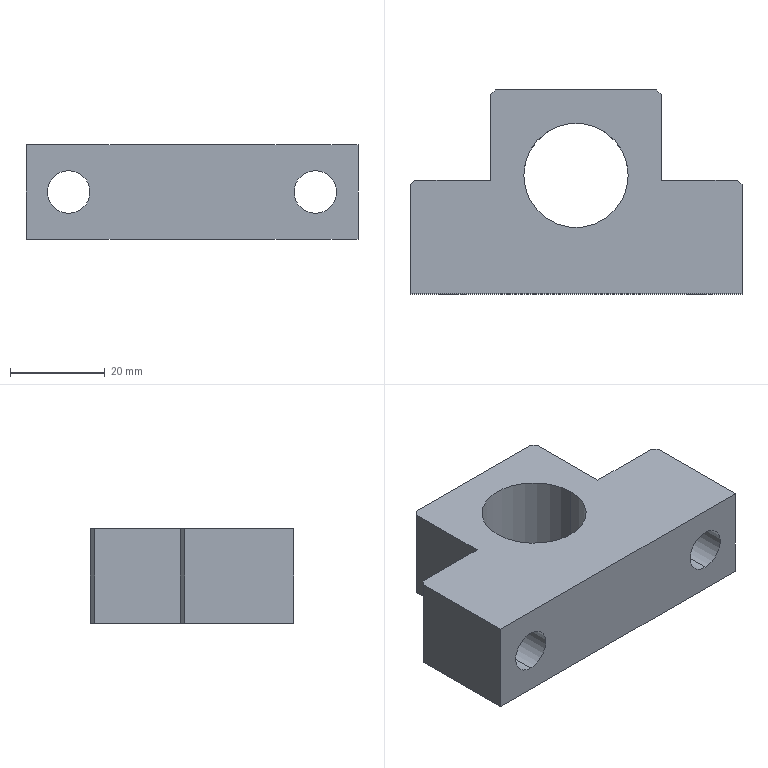Part | SolidWorks | features BaseBody 1 | 1 solid | 20 faces | box 70 x 43 x 20 mm | volume 36584 mm3 | plane 14 | cylinder 6 | commonest cylinder face diameters 9 x4 22 x2
STEP:
#1=CARTESIAN_POINT('',(-11.,0.,-10.));
#2=VERTEX_POINT('',#1);
#3=CARTESIAN_POINT('',(11.,0.,-10.));
#4=VERTEX_POINT('',#3);
#5=CARTESIAN_POINT('',(0.,0.,-10.));
#6=DIRECTION('',(0.,0.,1.));
#7=DIRECTION('',(1.,0.,0.));
#8=AXIS2_PLACEMENT_3D('',#5,#6,#7);
#9=CIRCLE('',#8,11.);
#10=EDGE_CURVE('',#2,#4,#9,.T.);
#11=ORIENTED_EDGE('',*,*,#10,.F.);
#12=CARTESIAN_POINT('',(-11.,0.,10.));
#13=VERTEX_POINT('',#12);
#14=CARTESIAN_POINT('',(-11.,0.,10.));
#15=DIRECTION('',(0.,0.,1.));
#16=VECTOR('',#15,1000.);
#17=LINE('',#14,#16);
#18=EDGE_CURVE('',#2,#13,#17,.T.);
#19=ORIENTED_EDGE('',*,*,#18,.T.);
#20=CARTESIAN_POINT('',(11.,0.,10.));
#21=VERTEX_POINT('',#20);
#22=CARTESIAN_POINT('',(0.,0.,10.));
#23=DIRECTION('',(0.,0.,1.));
#24=DIRECTION('',(1.,0.,0.));
#25=AXIS2_PLACEMENT_3D('',#22,#23,#24);
#26=CIRCLE('',#25,11.);
#27=EDGE_CURVE('',#13,#21,#26,.T.);
#28=ORIENTED_EDGE('',*,*,#27,.T.);
#29=CARTESIAN_POINT('',(11.,0.,10.));
#30=DIRECTION('',(0.,0.,1.));
#31=VECTOR('',#30,1000.);
#32=LINE('',#29,#31);
#33=EDGE_CURVE('',#4,#21,#32,.T.);
#34=ORIENTED_EDGE('',*,*,#33,.F.);
#35=EDGE_LOOP('',(#11,#19,#28,#34));
#36=FACE_OUTER_BOUND('',#35,.T.);
#37=CARTESIAN_POINT('',(0.,0.,10.));
#38=DIRECTION('',(0.,0.,1.));
#39=DIRECTION('',(1.,0.,0.));
#40=AXIS2_PLACEMENT_3D('',#37,#38,#39);
#41=CYLINDRICAL_SURFACE('',#40,11.);
#42=ADVANCED_FACE('',(#36),#41,.F.);
#43=CARTESIAN_POINT('',(26.,-25.,4.5));
#44=VERTEX_POINT('',#43);
#45=CARTESIAN_POINT('',(26.,-25.,-4.5));
#46=VERTEX_POINT('',#45);
#47=CARTESIAN_POINT('',(26.,-25.,0.));
#48=DIRECTION('',(0.,-1.,0.));
#49=DIRECTION('',(0.,0.,1.));
#50=AXIS2_PLACEMENT_3D('',#47,#48,#49);
#51=CIRCLE('',#50,4.5);
#52=EDGE_CURVE('',#44,#46,#51,.T.);
#53=ORIENTED_EDGE('',*,*,#52,.T.);
#54=CARTESIAN_POINT('',(26.,-1.,-4.5));
#55=VERTEX_POINT('',#54);
#56=CARTESIAN_POINT('',(26.,-25.,-4.5));
#57=DIRECTION('',(0.,1.,0.));
#58=VECTOR('',#57,1000.);
#59=LINE('',#56,#58);
#60=EDGE_CURVE('',#46,#55,#59,.T.);
#61=ORIENTED_EDGE('',*,*,#60,.T.);
#62=CARTESIAN_POINT('',(26.,-1.,4.5));
#63=VERTEX_POINT('',#62);
#64=CARTESIAN_POINT('',(26.,-1.,0.));
#65=DIRECTION('',(0.,1.,0.));
#66=DIRECTION('',(0.,0.,1.));
#67=AXIS2_PLACEMENT_3D('',#64,#65,#66);
#68=CIRCLE('',#67,4.5);
#69=EDGE_CURVE('',#55,#63,#68,.T.);
#70=ORIENTED_EDGE('',*,*,#69,.T.);
#71=CARTESIAN_POINT('',(26.,-25.,4.5));
#72=DIRECTION('',(0.,1.,0.));
#73=VECTOR('',#72,1000.);
#74=LINE('',#71,#73);
#75=EDGE_CURVE('',#44,#63,#74,.T.);
#76=ORIENTED_EDGE('',*,*,#75,.F.);
#77=EDGE_LOOP('',(#53,#61,#70,#76));
#78=FACE_OUTER_BOUND('',#77,.T.);
#79=CARTESIAN_POINT('',(26.,-25.,0.));
#80=DIRECTION('',(0.,1.,0.));
#81=DIRECTION('',(0.,0.,1.));
#82=AXIS2_PLACEMENT_3D('',#79,#80,#81);
#83=CYLINDRICAL_SURFACE('',#82,4.5);
#84=ADVANCED_FACE('',(#78),#83,.F.);
#85=CARTESIAN_POINT('',(-26.,-1.,-4.5));
#86=VERTEX_POINT('',#85);
#87=CARTESIAN_POINT('',(-26.,-1.,4.5));
#88=VERTEX_POINT('',#87);
#89=CARTESIAN_POINT('',(-26.,-1.,0.));
#90=DIRECTION('',(0.,1.,0.));
#91=DIRECTION('',(0.,0.,-1.));
#92=AXIS2_PLACEMENT_3D('',#89,#90,#91);
#93=CIRCLE('',#92,4.5);
#94=EDGE_CURVE('',#86,#88,#93,.T.);
#95=ORIENTED_EDGE('',*,*,#94,.T.);
#96=CARTESIAN_POINT('',(-26.,-25.,4.5));
#97=VERTEX_POINT('',#96);
#98=CARTESIAN_POINT('',(-26.,-1.,4.5));
#99=DIRECTION('',(0.,-1.,0.));
#100=VECTOR('',#99,1000.);
#101=LINE('',#98,#100);
#102=EDGE_CURVE('',#88,#97,#101,.T.);
#103=ORIENTED_EDGE('',*,*,#102,.T.);
#104=CARTESIAN_POINT('',(-26.,-25.,-4.5));
#105=VERTEX_POINT('',#104);
#106=CARTESIAN_POINT('',(-26.,-25.,0.));
#107=DIRECTION('',(0.,-1.,0.));
#108=DIRECTION('',(0.,0.,-1.));
#109=AXIS2_PLACEMENT_3D('',#106,#107,#108);
#110=CIRCLE('',#109,4.5);
#111=EDGE_CURVE('',#97,#105,#110,.T.);
#112=ORIENTED_EDGE('',*,*,#111,.T.);
#113=CARTESIAN_POINT('',(-26.,-1.,-4.5));
#114=DIRECTION('',(0.,-1.,0.));
#115=VECTOR('',#114,1000.);
#116=LINE('',#113,#115);
#117=EDGE_CURVE('',#86,#105,#116,.T.);
#118=ORIENTED_EDGE('',*,*,#117,.F.);
#119=EDGE_LOOP('',(#95,#103,#112,#118));
#120=FACE_OUTER_BOUND('',#119,.T.);
#121=CARTESIAN_POINT('',(-26.,-1.,0.));
#122=DIRECTION('',(0.,-1.,0.));
#123=DIRECTION('',(0.,0.,-1.));
#124=AXIS2_PLACEMENT_3D('',#121,#122,#123);
#125=CYLINDRICAL_SURFACE('',#124,4.5);
#126=ADVANCED_FACE('',(#120),#125,.F.);
#127=CARTESIAN_POINT('',(-35.,-25.,10.));
#128=VERTEX_POINT('',#127);
#129=CARTESIAN_POINT('',(-35.,-2.,10.));
#130=VERTEX_POINT('',#129);
#131=CARTESIAN_POINT('',(-35.,0.,10.));
#132=DIRECTION('',(0.,1.,0.));
#133=VECTOR('',#132,1000.);
#134=LINE('',#131,#133);
#135=EDGE_CURVE('',#128,#130,#134,.T.);
#136=ORIENTED_EDGE('',*,*,#135,.F.);
#137=CARTESIAN_POINT('',(35.,-25.,10.));
#138=VERTEX_POINT('',#137);
#139=CARTESIAN_POINT('',(0.,-25.,10.));
#140=DIRECTION('',(-1.,0.,0.));
#141=VECTOR('',#140,1000.);
#142=LINE('',#139,#141);
#143=EDGE_CURVE('',#138,#128,#142,.T.);
#144=ORIENTED_EDGE('',*,*,#143,.F.);
#145=CARTESIAN_POINT('',(35.,-2.,10.));
#146=VERTEX_POINT('',#145);
#147=CARTESIAN_POINT('',(35.,0.,10.));
#148=DIRECTION('',(0.,-1.,0.));
#149=VECTOR('',#148,1000.);
#150=LINE('',#147,#149);
#151=EDGE_CURVE('',#146,#138,#150,.T.);
#152=ORIENTED_EDGE('',*,*,#151,.F.);
#153=CARTESIAN_POINT('',(34.,-1.,10.));
#154=VERTEX_POINT('',#153);
#155=CARTESIAN_POINT('',(35.,-2.,10.));
#156=DIRECTION('',(-0.7071,0.7071,0.));
#157=VECTOR('',#156,1000.);
#158=LINE('',#155,#157);
#159=EDGE_CURVE('',#146,#154,#158,.T.);
#160=ORIENTED_EDGE('',*,*,#159,.T.);
#161=CARTESIAN_POINT('',(18.,-1.,10.));
#162=VERTEX_POINT('',#161);
#163=CARTESIAN_POINT('',(0.,-1.,10.));
#164=DIRECTION('',(1.,0.,0.));
#165=VECTOR('',#164,1000.);
#166=LINE('',#163,#165);
#167=EDGE_CURVE('',#162,#154,#166,.T.);
#168=ORIENTED_EDGE('',*,*,#167,.F.);
#169=CARTESIAN_POINT('',(18.,17.,10.));
#170=VERTEX_POINT('',#169);
#171=CARTESIAN_POINT('',(18.,0.,10.));
#172=DIRECTION('',(0.,-1.,0.));
#173=VECTOR('',#172,1000.);
#174=LINE('',#171,#173);
#175=EDGE_CURVE('',#170,#162,#174,.T.);
#176=ORIENTED_EDGE('',*,*,#175,.F.);
#177=CARTESIAN_POINT('',(17.,18.,10.));
#178=VERTEX_POINT('',#177);
#179=CARTESIAN_POINT('',(18.,17.,10.));
#180=DIRECTION('',(-0.7071,0.7071,0.));
#181=VECTOR('',#180,1000.);
#182=LINE('',#179,#181);
#183=EDGE_CURVE('',#170,#178,#182,.T.);
#184=ORIENTED_EDGE('',*,*,#183,.T.);
#185=CARTESIAN_POINT('',(-17.,18.,10.));
#186=VERTEX_POINT('',#185);
#187=CARTESIAN_POINT('',(0.,18.,10.));
#188=DIRECTION('',(1.,0.,0.));
#189=VECTOR('',#188,1000.);
#190=LINE('',#187,#189);
#191=EDGE_CURVE('',#186,#178,#190,.T.);
#192=ORIENTED_EDGE('',*,*,#191,.F.);
#193=CARTESIAN_POINT('',(-18.,17.,10.));
#194=VERTEX_POINT('',#193);
#195=CARTESIAN_POINT('',(-17.,18.,10.));
#196=DIRECTION('',(-0.7071,-0.7071,0.));
#197=VECTOR('',#196,1000.);
#198=LINE('',#195,#197);
#199=EDGE_CURVE('',#186,#194,#198,.T.);
#200=ORIENTED_EDGE('',*,*,#199,.T.);
#201=CARTESIAN_POINT('',(-18.,-1.,10.));
#202=VERTEX_POINT('',#201);
#203=CARTESIAN_POINT('',(-18.,0.,10.));
#204=DIRECTION('',(0.,1.,0.));
#205=VECTOR('',#204,1000.);
#206=LINE('',#203,#205);
#207=EDGE_CURVE('',#202,#194,#206,.T.);
#208=ORIENTED_EDGE('',*,*,#207,.F.);
#209=CARTESIAN_POINT('',(-34.,-1.,10.));
#210=VERTEX_POINT('',#209);
#211=CARTESIAN_POINT('',(0.,-1.,10.));
#212=DIRECTION('',(1.,0.,0.));
#213=VECTOR('',#212,1000.);
#214=LINE('',#211,#213);
#215=EDGE_CURVE('',#210,#202,#214,.T.);
#216=ORIENTED_EDGE('',*,*,#215,.F.);
#217=CARTESIAN_POINT('',(-34.,-1.,10.));
#218=DIRECTION('',(-0.7071,-0.7071,0.));
#219=VECTOR('',#218,1000.);
#220=LINE('',#217,#219);
#221=EDGE_CURVE('',#210,#130,#220,.T.);
#222=ORIENTED_EDGE('',*,*,#221,.T.);
#223=EDGE_LOOP('',(#136,#144,#152,#160,#168,#176,#184,#192,#200,#208,#216,#222));
#224=FACE_OUTER_BOUND('',#223,.T.);
#225=CARTESIAN_POINT('',(0.,0.,10.));
#226=DIRECTION('',(0.,0.,1.));
#227=DIRECTION('',(1.,0.,0.));
#228=AXIS2_PLACEMENT_3D('',#225,#226,#227);
#229=CIRCLE('',#228,11.);
#230=EDGE_CURVE('',#21,#13,#229,.T.);
#231=ORIENTED_EDGE('',*,*,#230,.F.);
#232=ORIENTED_EDGE('',*,*,#27,.F.);
#233=EDGE_LOOP('',(#231,#232));
#234=FACE_BOUND('',#233,.T.);
#235=CARTESIAN_POINT('',(0.,0.,10.));
#236=DIRECTION('',(0.,0.,-1.));
#237=DIRECTION('',(-1.,0.,0.));
#238=AXIS2_PLACEMENT_3D('',#235,#236,#237);
#239=PLANE('',#238);
#240=ADVANCED_FACE('',(#224,#234),#239,.F.);
#241=CARTESIAN_POINT('',(-35.,-25.,-10.));
#242=VERTEX_POINT('',#241);
#243=CARTESIAN_POINT('',(-35.,-25.,10.));
#244=DIRECTION('',(0.,0.,-1.));
#245=VECTOR('',#244,1000.);
#246=LINE('',#243,#245);
#247=EDGE_CURVE('',#128,#242,#246,.T.);
#248=ORIENTED_EDGE('',*,*,#247,.F.);
#249=ORIENTED_EDGE('',*,*,#135,.T.);
#250=CARTESIAN_POINT('',(-35.,-2.,-10.));
#251=VERTEX_POINT('',#250);
#252=CARTESIAN_POINT('',(-35.,-2.,10.));
#253=DIRECTION('',(0.,0.,1.));
#254=VECTOR('',#253,1000.);
#255=LINE('',#252,#254);
#256=EDGE_CURVE('',#251,#130,#255,.T.);
#257=ORIENTED_EDGE('',*,*,#256,.F.);
#258=CARTESIAN_POINT('',(-35.,-2.,-10.));
#259=DIRECTION('',(0.,1.,0.));
#260=VECTOR('',#259,1000.);
#261=LINE('',#258,#260);
#262=EDGE_CURVE('',#242,#251,#261,.T.);
#263=ORIENTED_EDGE('',*,*,#262,.F.);
#264=EDGE_LOOP('',(#248,#249,#257,#263));
#265=FACE_OUTER_BOUND('',#264,.T.);
#266=CARTESIAN_POINT('',(-35.,-2.,10.));
#267=DIRECTION('',(1.,0.,0.));
#268=DIRECTION('',(0.,0.,-1.));
#269=AXIS2_PLACEMENT_3D('',#266,#267,#268);
#270=PLANE('',#269);
#271=ADVANCED_FACE('',(#265),#270,.F.);
#272=CARTESIAN_POINT('',(35.,-25.,-10.));
#273=VERTEX_POINT('',#272);
#274=CARTESIAN_POINT('',(35.,-25.,10.));
#275=DIRECTION('',(0.,0.,-1.));
#276=VECTOR('',#275,1000.);
#277=LINE('',#274,#276);
#278=EDGE_CURVE('',#138,#273,#277,.T.);
#279=ORIENTED_EDGE('',*,*,#278,.F.);
#280=ORIENTED_EDGE('',*,*,#143,.T.);
#281=ORIENTED_EDGE('',*,*,#247,.T.);
#282=CARTESIAN_POINT('',(-35.,-25.,-10.));
#283=DIRECTION('',(-1.,0.,0.));
#284=VECTOR('',#283,1000.);
#285=LINE('',#282,#284);
#286=EDGE_CURVE('',#273,#242,#285,.T.);
#287=ORIENTED_EDGE('',*,*,#286,.F.);
#288=EDGE_LOOP('',(#279,#280,#281,#287));
#289=FACE_OUTER_BOUND('',#288,.T.);
#290=ORIENTED_EDGE('',*,*,#52,.F.);
#291=CARTESIAN_POINT('',(26.,-25.,0.));
#292=DIRECTION('',(0.,-1.,0.));
#293=DIRECTION('',(0.,0.,1.));
#294=AXIS2_PLACEMENT_3D('',#291,#292,#293);
#295=CIRCLE('',#294,4.5);
#296=EDGE_CURVE('',#46,#44,#295,.T.);
#297=ORIENTED_EDGE('',*,*,#296,.F.);
#298=EDGE_LOOP('',(#290,#297));
#299=FACE_BOUND('',#298,.T.);
#300=CARTESIAN_POINT('',(-26.,-25.,0.));
#301=DIRECTION('',(0.,-1.,0.));
#302=DIRECTION('',(0.,0.,-1.));
#303=AXIS2_PLACEMENT_3D('',#300,#301,#302);
#304=CIRCLE('',#303,4.5);
#305=EDGE_CURVE('',#105,#97,#304,.T.);
#306=ORIENTED_EDGE('',*,*,#305,.F.);
#307=ORIENTED_EDGE('',*,*,#111,.F.);
#308=EDGE_LOOP('',(#306,#307));
#309=FACE_BOUND('',#308,.T.);
#310=CARTESIAN_POINT('',(-35.,-25.,10.));
#311=DIRECTION('',(0.,1.,0.));
#312=DIRECTION('',(0.,0.,1.));
#313=AXIS2_PLACEMENT_3D('',#310,#311,#312);
#314=PLANE('',#313);
#315=ADVANCED_FACE('',(#289,#299,#309),#314,.F.);
#316=CARTESIAN_POINT('',(35.,-2.,-10.));
#317=VERTEX_POINT('',#316);
#318=CARTESIAN_POINT('',(35.,-2.,10.));
#319=DIRECTION('',(0.,0.,-1.));
#320=VECTOR('',#319,1000.);
#321=LINE('',#318,#320);
#322=EDGE_CURVE('',#146,#317,#321,.T.);
#323=ORIENTED_EDGE('',*,*,#322,.F.);
#324=ORIENTED_EDGE('',*,*,#151,.T.);
#325=ORIENTED_EDGE('',*,*,#278,.T.);
#326=CARTESIAN_POINT('',(35.,-25.,-10.));
#327=DIRECTION('',(0.,-1.,0.));
#328=VECTOR('',#327,1000.);
#329=LINE('',#326,#328);
#330=EDGE_CURVE('',#317,#273,#329,.T.);
#331=ORIENTED_EDGE('',*,*,#330,.F.);
#332=EDGE_LOOP('',(#323,#324,#325,#331));
#333=FACE_OUTER_BOUND('',#332,.T.);
#334=CARTESIAN_POINT('',(35.,-25.,10.));
#335=DIRECTION('',(-1.,0.,0.));
#336=DIRECTION('',(0.,0.,1.));
#337=AXIS2_PLACEMENT_3D('',#334,#335,#336);
#338=PLANE('',#337);
#339=ADVANCED_FACE('',(#333),#338,.F.);
#340=CARTESIAN_POINT('',(18.,-1.,-10.));
#341=VERTEX_POINT('',#340);
#342=CARTESIAN_POINT('',(18.,-1.,10.));
#343=DIRECTION('',(0.,0.,-1.));
#344=VECTOR('',#343,1000.);
#345=LINE('',#342,#344);
#346=EDGE_CURVE('',#162,#341,#345,.T.);
#347=ORIENTED_EDGE('',*,*,#346,.F.);
#348=ORIENTED_EDGE('',*,*,#167,.T.);
#349=CARTESIAN_POINT('',(34.,-1.,-10.));
#350=VERTEX_POINT('',#349);
#351=CARTESIAN_POINT('',(34.,-1.,10.));
#352=DIRECTION('',(0.,0.,1.));
#353=VECTOR('',#352,1000.);
#354=LINE('',#351,#353);
#355=EDGE_CURVE('',#350,#154,#354,.T.);
#356=ORIENTED_EDGE('',*,*,#355,.F.);
#357=CARTESIAN_POINT('',(34.,-1.,-10.));
#358=DIRECTION('',(1.,0.,0.));
#359=VECTOR('',#358,1000.);
#360=LINE('',#357,#359);
#361=EDGE_CURVE('',#341,#350,#360,.T.);
#362=ORIENTED_EDGE('',*,*,#361,.F.);
#363=EDGE_LOOP('',(#347,#348,#356,#362));
#364=FACE_OUTER_BOUND('',#363,.T.);
#365=CARTESIAN_POINT('',(26.,-1.,0.));
#366=DIRECTION('',(0.,1.,0.));
#367=DIRECTION('',(0.,0.,1.));
#368=AXIS2_PLACEMENT_3D('',#365,#366,#367);
#369=CIRCLE('',#368,4.5);
#370=EDGE_CURVE('',#63,#55,#369,.T.);
#371=ORIENTED_EDGE('',*,*,#370,.F.);
#372=ORIENTED_EDGE('',*,*,#69,.F.);
#373=EDGE_LOOP('',(#371,#372));
#374=FACE_BOUND('',#373,.T.);
#375=CARTESIAN_POINT('',(34.,-1.,10.));
#376=DIRECTION('',(0.,-1.,0.));
#377=DIRECTION('',(0.,0.,-1.));
#378=AXIS2_PLACEMENT_3D('',#375,#376,#377);
#379=PLANE('',#378);
#380=ADVANCED_FACE('',(#364,#374),#379,.F.);
#381=CARTESIAN_POINT('',(18.,17.,-10.));
#382=VERTEX_POINT('',#381);
#383=CARTESIAN_POINT('',(18.,17.,10.));
#384=DIRECTION('',(0.,0.,-1.));
#385=VECTOR('',#384,1000.);
#386=LINE('',#383,#385);
#387=EDGE_CURVE('',#170,#382,#386,.T.);
#388=ORIENTED_EDGE('',*,*,#387,.F.);
#389=ORIENTED_EDGE('',*,*,#175,.T.);
#390=ORIENTED_EDGE('',*,*,#346,.T.);
#391=CARTESIAN_POINT('',(18.,-1.,-10.));
#392=DIRECTION('',(0.,-1.,0.));
#393=VECTOR('',#392,1000.);
#394=LINE('',#391,#393);
#395=EDGE_CURVE('',#382,#341,#394,.T.);
#396=ORIENTED_EDGE('',*,*,#395,.F.);
#397=EDGE_LOOP('',(#388,#389,#390,#396));
#398=FACE_OUTER_BOUND('',#397,.T.);
#399=CARTESIAN_POINT('',(18.,-1.,10.));
#400=DIRECTION('',(-1.,0.,0.));
#401=DIRECTION('',(0.,0.,1.));
#402=AXIS2_PLACEMENT_3D('',#399,#400,#401);
#403=PLANE('',#402);
#404=ADVANCED_FACE('',(#398),#403,.F.);
#405=CARTESIAN_POINT('',(-17.,18.,-10.));
#406=VERTEX_POINT('',#405);
#407=CARTESIAN_POINT('',(-17.,18.,10.));
#408=DIRECTION('',(0.,0.,-1.));
#409=VECTOR('',#408,1000.);
#410=LINE('',#407,#409);
#411=EDGE_CURVE('',#186,#406,#410,.T.);
#412=ORIENTED_EDGE('',*,*,#411,.F.);
#413=ORIENTED_EDGE('',*,*,#191,.T.);
#414=CARTESIAN_POINT('',(17.,18.,-10.));
#415=VERTEX_POINT('',#414);
#416=CARTESIAN_POINT('',(17.,18.,10.));
#417=DIRECTION('',(0.,0.,1.));
#418=VECTOR('',#417,1000.);
#419=LINE('',#416,#418);
#420=EDGE_CURVE('',#415,#178,#419,.T.);
#421=ORIENTED_EDGE('',*,*,#420,.F.);
#422=CARTESIAN_POINT('',(17.,18.,-10.));
#423=DIRECTION('',(1.,0.,0.));
#424=VECTOR('',#423,1000.);
#425=LINE('',#422,#424);
#426=EDGE_CURVE('',#406,#415,#425,.T.);
#427=ORIENTED_EDGE('',*,*,#426,.F.);
#428=EDGE_LOOP('',(#412,#413,#421,#427));
#429=FACE_OUTER_BOUND('',#428,.T.);
#430=CARTESIAN_POINT('',(17.,18.,10.));
#431=DIRECTION('',(0.,-1.,0.));
#432=DIRECTION('',(0.,0.,-1.));
#433=AXIS2_PLACEMENT_3D('',#430,#431,#432);
#434=PLANE('',#433);
#435=ADVANCED_FACE('',(#429),#434,.F.);
#436=CARTESIAN_POINT('',(-18.,-1.,-10.));
#437=VERTEX_POINT('',#436);
#438=CARTESIAN_POINT('',(-18.,-1.,10.));
#439=DIRECTION('',(0.,0.,-1.));
#440=VECTOR('',#439,1000.);
#441=LINE('',#438,#440);
#442=EDGE_CURVE('',#202,#437,#441,.T.);
#443=ORIENTED_EDGE('',*,*,#442,.F.);
#444=ORIENTED_EDGE('',*,*,#207,.T.);
#445=CARTESIAN_POINT('',(-18.,17.,-10.));
#446=VERTEX_POINT('',#445);
#447=CARTESIAN_POINT('',(-18.,17.,10.));
#448=DIRECTION('',(0.,0.,1.));
#449=VECTOR('',#448,1000.);
#450=LINE('',#447,#449);
#451=EDGE_CURVE('',#446,#194,#450,.T.);
#452=ORIENTED_EDGE('',*,*,#451,.F.);
#453=CARTESIAN_POINT('',(-18.,17.,-10.));
#454=DIRECTION('',(0.,1.,0.));
#455=VECTOR('',#454,1000.);
#456=LINE('',#453,#455);
#457=EDGE_CURVE('',#437,#446,#456,.T.);
#458=ORIENTED_EDGE('',*,*,#457,.F.);
#459=EDGE_LOOP('',(#443,#444,#452,#458));
#460=FACE_OUTER_BOUND('',#459,.T.);
#461=CARTESIAN_POINT('',(-18.,17.,10.));
#462=DIRECTION('',(1.,0.,0.));
#463=DIRECTION('',(0.,0.,-1.));
#464=AXIS2_PLACEMENT_3D('',#461,#462,#463);
#465=PLANE('',#464);
#466=ADVANCED_FACE('',(#460),#465,.F.);
#467=CARTESIAN_POINT('',(-34.,-1.,-10.));
#468=VERTEX_POINT('',#467);
#469=CARTESIAN_POINT('',(-34.,-1.,10.));
#470=DIRECTION('',(0.,0.,-1.));
#471=VECTOR('',#470,1000.);
#472=LINE('',#469,#471);
#473=EDGE_CURVE('',#210,#468,#472,.T.);
#474=ORIENTED_EDGE('',*,*,#473,.F.);
#475=ORIENTED_EDGE('',*,*,#215,.T.);
#476=ORIENTED_EDGE('',*,*,#442,.T.);
#477=CARTESIAN_POINT('',(-18.,-1.,-10.));
#478=DIRECTION('',(1.,0.,0.));
#479=VECTOR('',#478,1000.);
#480=LINE('',#477,#479);
#481=EDGE_CURVE('',#468,#437,#480,.T.);
#482=ORIENTED_EDGE('',*,*,#481,.F.);
#483=EDGE_LOOP('',(#474,#475,#476,#482));
#484=FACE_OUTER_BOUND('',#483,.T.);
#485=ORIENTED_EDGE('',*,*,#94,.F.);
#486=CARTESIAN_POINT('',(-26.,-1.,0.));
#487=DIRECTION('',(0.,1.,0.));
#488=DIRECTION('',(0.,0.,-1.));
#489=AXIS2_PLACEMENT_3D('',#486,#487,#488);
#490=CIRCLE('',#489,4.5);
#491=EDGE_CURVE('',#88,#86,#490,.T.);
#492=ORIENTED_EDGE('',*,*,#491,.F.);
#493=EDGE_LOOP('',(#485,#492));
#494=FACE_BOUND('',#493,.T.);
#495=CARTESIAN_POINT('',(-18.,-1.,10.));
#496=DIRECTION('',(0.,-1.,0.));
#497=DIRECTION('',(0.,0.,-1.));
#498=AXIS2_PLACEMENT_3D('',#495,#496,#497);
#499=PLANE('',#498);
#500=ADVANCED_FACE('',(#484,#494),#499,.F.);
#501=ORIENTED_EDGE('',*,*,#18,.F.);
#502=CARTESIAN_POINT('',(0.,0.,-10.));
#503=DIRECTION('',(0.,0.,1.));
#504=DIRECTION('',(1.,0.,0.));
#505=AXIS2_PLACEMENT_3D('',#502,#503,#504);
#506=CIRCLE('',#505,11.);
#507=EDGE_CURVE('',#4,#2,#506,.T.);
#508=ORIENTED_EDGE('',*,*,#507,.F.);
#509=ORIENTED_EDGE('',*,*,#33,.T.);
#510=ORIENTED_EDGE('',*,*,#230,.T.);
#511=EDGE_LOOP('',(#501,#508,#509,#510));
#512=FACE_OUTER_BOUND('',#511,.T.);
#513=CARTESIAN_POINT('',(0.,0.,10.));
#514=DIRECTION('',(0.,0.,1.));
#515=DIRECTION('',(1.,0.,0.));
#516=AXIS2_PLACEMENT_3D('',#513,#514,#515);
#517=CYLINDRICAL_SURFACE('',#516,11.);
#518=ADVANCED_FACE('',(#512),#517,.F.);
#519=ORIENTED_EDGE('',*,*,#286,.T.);
#520=ORIENTED_EDGE('',*,*,#262,.T.);
#521=CARTESIAN_POINT('',(-35.,-2.,-10.));
#522=DIRECTION('',(0.7071,0.7071,0.));
#523=VECTOR('',#522,1000.);
#524=LINE('',#521,#523);
#525=EDGE_CURVE('',#251,#468,#524,.T.);
#526=ORIENTED_EDGE('',*,*,#525,.T.);
#527=ORIENTED_EDGE('',*,*,#481,.T.);
#528=ORIENTED_EDGE('',*,*,#457,.T.);
#529=CARTESIAN_POINT('',(-18.,17.,-10.));
#530=DIRECTION('',(0.7071,0.7071,0.));
#531=VECTOR('',#530,1000.);
#532=LINE('',#529,#531);
#533=EDGE_CURVE('',#446,#406,#532,.T.);
#534=ORIENTED_EDGE('',*,*,#533,.T.);
#535=ORIENTED_EDGE('',*,*,#426,.T.);
#536=CARTESIAN_POINT('',(17.,18.,-10.));
#537=DIRECTION('',(0.7071,-0.7071,0.));
#538=VECTOR('',#537,1000.);
#539=LINE('',#536,#538);
#540=EDGE_CURVE('',#415,#382,#539,.T.);
#541=ORIENTED_EDGE('',*,*,#540,.T.);
#542=ORIENTED_EDGE('',*,*,#395,.T.);
#543=ORIENTED_EDGE('',*,*,#361,.T.);
#544=CARTESIAN_POINT('',(34.,-1.,-10.));
#545=DIRECTION('',(0.7071,-0.7071,0.));
#546=VECTOR('',#545,1000.);
#547=LINE('',#544,#546);
#548=EDGE_CURVE('',#350,#317,#547,.T.);
#549=ORIENTED_EDGE('',*,*,#548,.T.);
#550=ORIENTED_EDGE('',*,*,#330,.T.);
#551=EDGE_LOOP('',(#519,#520,#526,#527,#528,#534,#535,#541,#542,#543,#549,#550));
#552=FACE_OUTER_BOUND('',#551,.T.);
#553=ORIENTED_EDGE('',*,*,#507,.T.);
#554=ORIENTED_EDGE('',*,*,#10,.T.);
#555=EDGE_LOOP('',(#553,#554));
#556=FACE_BOUND('',#555,.T.);
#557=CARTESIAN_POINT('',(0.,0.,-10.));
#558=DIRECTION('',(0.,0.,-1.));
#559=DIRECTION('',(-1.,0.,0.));
#560=AXIS2_PLACEMENT_3D('',#557,#558,#559);
#561=PLANE('',#560);
#562=ADVANCED_FACE('',(#552,#556),#561,.T.);
#563=ORIENTED_EDGE('',*,*,#256,.T.);
#564=ORIENTED_EDGE('',*,*,#221,.F.);
#565=ORIENTED_EDGE('',*,*,#473,.T.);
#566=ORIENTED_EDGE('',*,*,#525,.F.);
#567=EDGE_LOOP('',(#563,#564,#565,#566));
#568=FACE_OUTER_BOUND('',#567,.T.);
#569=CARTESIAN_POINT('',(-34.,-1.,10.));
#570=DIRECTION('',(0.7071,-0.7071,0.));
#571=DIRECTION('',(0.7071,0.7071,0.));
#572=AXIS2_PLACEMENT_3D('',#569,#570,#571);
#573=PLANE('',#572);
#574=ADVANCED_FACE('',(#568),#573,.F.);
#575=ORIENTED_EDGE('',*,*,#60,.F.);
#576=ORIENTED_EDGE('',*,*,#296,.T.);
#577=ORIENTED_EDGE('',*,*,#75,.T.);
#578=ORIENTED_EDGE('',*,*,#370,.T.);
#579=EDGE_LOOP('',(#575,#576,#577,#578));
#580=FACE_OUTER_BOUND('',#579,.T.);
#581=CARTESIAN_POINT('',(26.,-25.,0.));
#582=DIRECTION('',(0.,1.,0.));
#583=DIRECTION('',(0.,0.,1.));
#584=AXIS2_PLACEMENT_3D('',#581,#582,#583);
#585=CYLINDRICAL_SURFACE('',#584,4.5);
#586=ADVANCED_FACE('',(#580),#585,.F.);
#587=ORIENTED_EDGE('',*,*,#102,.F.);
#588=ORIENTED_EDGE('',*,*,#491,.T.);
#589=ORIENTED_EDGE('',*,*,#117,.T.);
#590=ORIENTED_EDGE('',*,*,#305,.T.);
#591=EDGE_LOOP('',(#587,#588,#589,#590));
#592=FACE_OUTER_BOUND('',#591,.T.);
#593=CARTESIAN_POINT('',(-26.,-1.,0.));
#594=DIRECTION('',(0.,-1.,0.));
#595=DIRECTION('',(0.,0.,-1.));
#596=AXIS2_PLACEMENT_3D('',#593,#594,#595);
#597=CYLINDRICAL_SURFACE('',#596,4.5);
#598=ADVANCED_FACE('',(#592),#597,.F.);
#599=ORIENTED_EDGE('',*,*,#355,.T.);
#600=ORIENTED_EDGE('',*,*,#159,.F.);
#601=ORIENTED_EDGE('',*,*,#322,.T.);
#602=ORIENTED_EDGE('',*,*,#548,.F.);
#603=EDGE_LOOP('',(#599,#600,#601,#602));
#604=FACE_OUTER_BOUND('',#603,.T.);
#605=CARTESIAN_POINT('',(35.,-2.,10.));
#606=DIRECTION('',(-0.7071,-0.7071,0.));
#607=DIRECTION('',(0.7071,-0.7071,0.));
#608=AXIS2_PLACEMENT_3D('',#605,#606,#607);
#609=PLANE('',#608);
#610=ADVANCED_FACE('',(#604),#609,.F.);
#611=ORIENTED_EDGE('',*,*,#420,.T.);
#612=ORIENTED_EDGE('',*,*,#183,.F.);
#613=ORIENTED_EDGE('',*,*,#387,.T.);
#614=ORIENTED_EDGE('',*,*,#540,.F.);
#615=EDGE_LOOP('',(#611,#612,#613,#614));
#616=FACE_OUTER_BOUND('',#615,.T.);
#617=CARTESIAN_POINT('',(18.,17.,10.));
#618=DIRECTION('',(-0.7071,-0.7071,0.));
#619=DIRECTION('',(0.7071,-0.7071,0.));
#620=AXIS2_PLACEMENT_3D('',#617,#618,#619);
#621=PLANE('',#620);
#622=ADVANCED_FACE('',(#616),#621,.F.);
#623=ORIENTED_EDGE('',*,*,#451,.T.);
#624=ORIENTED_EDGE('',*,*,#199,.F.);
#625=ORIENTED_EDGE('',*,*,#411,.T.);
#626=ORIENTED_EDGE('',*,*,#533,.F.);
#627=EDGE_LOOP('',(#623,#624,#625,#626));
#628=FACE_OUTER_BOUND('',#627,.T.);
#629=CARTESIAN_POINT('',(-17.,18.,10.));
#630=DIRECTION('',(0.7071,-0.7071,0.));
#631=DIRECTION('',(0.7071,0.7071,0.));
#632=AXIS2_PLACEMENT_3D('',#629,#630,#631);
#633=PLANE('',#632);
#634=ADVANCED_FACE('',(#628),#633,.F.);
#635=CLOSED_SHELL('',(#42,#84,#126,#240,#271,#315,#339,#380,#404,#435,#466,#500,#518,#562,#574,#586,#598,#610,#622,#634));
#636=MANIFOLD_SOLID_BREP('',#635);
#637=CARTESIAN_POINT('',(0.,0.,0.));
#638=DIRECTION('',(0.,0.,1.));
#639=DIRECTION('',(1.,0.,0.));
#640=AXIS2_PLACEMENT_3D('',#637,#638,#639);
#641=(LENGTH_UNIT()NAMED_UNIT(*)SI_UNIT(.MILLI.,.METRE.));
#642=UNCERTAINTY_MEASURE_WITH_UNIT(LENGTH_MEASURE(0.00001),#641,'','');
#643=(NAMED_UNIT(*)PLANE_ANGLE_UNIT()SI_UNIT($,.RADIAN.));
#644=(NAMED_UNIT(*)SI_UNIT($,.STERADIAN.)SOLID_ANGLE_UNIT());
#645=(GEOMETRIC_REPRESENTATION_CONTEXT(3)GLOBAL_UNCERTAINTY_ASSIGNED_CONTEXT((#642))GLOBAL_UNIT_ASSIGNED_CONTEXT((#641,#643,#644))REPRESENTATION_CONTEXT('',''));
#646=ADVANCED_BREP_SHAPE_REPRESENTATION('',(#636,#640),#645);